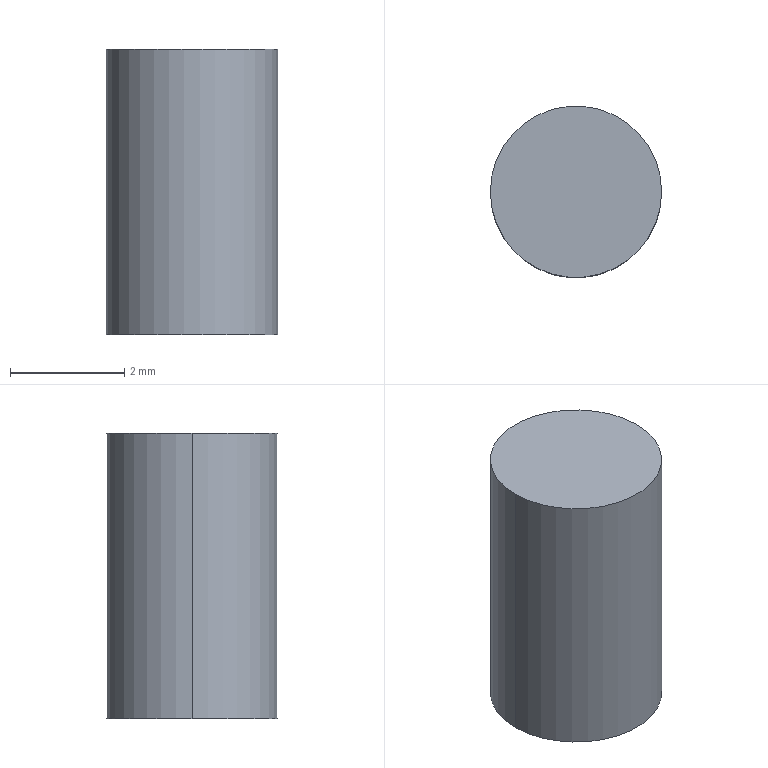Part | NX | features BREP 1 | 1 solid | 4 faces | box 3 x 3 x 5 mm | volume 35.343 mm3 | cylinder 2 | plane 2 | commonest cylinder face diameters 3 x2
STEP:
#1=CARTESIAN_POINT('',(1.5,0.,5.));
#2=VERTEX_POINT('',#1);
#3=CARTESIAN_POINT('',(-1.5,0.,5.));
#4=VERTEX_POINT('',#3);
#5=CARTESIAN_POINT('',(0.,0.,5.));
#6=DIRECTION('',(0.,0.,1.));
#7=DIRECTION('',(1.,0.,0.));
#8=AXIS2_PLACEMENT_3D('',#5,#6,#7);
#9=CIRCLE('',#8,1.5);
#10=EDGE_CURVE('',#2,#4,#9,.T.);
#11=ORIENTED_EDGE('',*,*,#10,.F.);
#12=CARTESIAN_POINT('',(1.5,0.,0.));
#13=VERTEX_POINT('',#12);
#14=CARTESIAN_POINT('',(1.5,0.,5.));
#15=DIRECTION('',(0.,0.,-1.));
#16=VECTOR('',#15,1000.);
#17=LINE('',#14,#16);
#18=EDGE_CURVE('',#2,#13,#17,.T.);
#19=ORIENTED_EDGE('',*,*,#18,.T.);
#20=CARTESIAN_POINT('',(-1.5,0.,0.));
#21=VERTEX_POINT('',#20);
#22=CARTESIAN_POINT('',(0.,0.,0.));
#23=DIRECTION('',(0.,0.,1.));
#24=DIRECTION('',(1.,0.,0.));
#25=AXIS2_PLACEMENT_3D('',#22,#23,#24);
#26=CIRCLE('',#25,1.5);
#27=EDGE_CURVE('',#13,#21,#26,.T.);
#28=ORIENTED_EDGE('',*,*,#27,.T.);
#29=CARTESIAN_POINT('',(-1.5,0.,5.));
#30=DIRECTION('',(0.,0.,-1.));
#31=VECTOR('',#30,1000.);
#32=LINE('',#29,#31);
#33=EDGE_CURVE('',#4,#21,#32,.T.);
#34=ORIENTED_EDGE('',*,*,#33,.F.);
#35=EDGE_LOOP('',(#11,#19,#28,#34));
#36=FACE_BOUND('',#35,.T.);
#37=CARTESIAN_POINT('',(0.,0.,5.));
#38=DIRECTION('',(0.,0.,-1.));
#39=DIRECTION('',(-1.,0.,0.));
#40=AXIS2_PLACEMENT_3D('',#37,#38,#39);
#41=CYLINDRICAL_SURFACE('',#40,1.5);
#42=ADVANCED_FACE('',(#36),#41,.T.);
#43=ORIENTED_EDGE('',*,*,#18,.F.);
#44=CARTESIAN_POINT('',(0.,0.,5.));
#45=DIRECTION('',(0.,0.,1.));
#46=DIRECTION('',(1.,0.,0.));
#47=AXIS2_PLACEMENT_3D('',#44,#45,#46);
#48=CIRCLE('',#47,1.5);
#49=EDGE_CURVE('',#4,#2,#48,.T.);
#50=ORIENTED_EDGE('',*,*,#49,.F.);
#51=ORIENTED_EDGE('',*,*,#33,.T.);
#52=CARTESIAN_POINT('',(0.,0.,0.));
#53=DIRECTION('',(0.,0.,1.));
#54=DIRECTION('',(1.,0.,0.));
#55=AXIS2_PLACEMENT_3D('',#52,#53,#54);
#56=CIRCLE('',#55,1.5);
#57=EDGE_CURVE('',#21,#13,#56,.T.);
#58=ORIENTED_EDGE('',*,*,#57,.T.);
#59=EDGE_LOOP('',(#43,#50,#51,#58));
#60=FACE_BOUND('',#59,.T.);
#61=CARTESIAN_POINT('',(0.,0.,5.));
#62=DIRECTION('',(0.,0.,-1.));
#63=DIRECTION('',(-1.,0.,0.));
#64=AXIS2_PLACEMENT_3D('',#61,#62,#63);
#65=CYLINDRICAL_SURFACE('',#64,1.5);
#66=ADVANCED_FACE('',(#60),#65,.T.);
#67=ORIENTED_EDGE('',*,*,#49,.T.);
#68=ORIENTED_EDGE('',*,*,#10,.T.);
#69=EDGE_LOOP('',(#67,#68));
#70=FACE_BOUND('',#69,.T.);
#71=CARTESIAN_POINT('',(0.,0.,5.));
#72=DIRECTION('',(0.,0.,1.));
#73=DIRECTION('',(1.,0.,0.));
#74=AXIS2_PLACEMENT_3D('',#71,#72,#73);
#75=PLANE('',#74);
#76=ADVANCED_FACE('',(#70),#75,.T.);
#77=ORIENTED_EDGE('',*,*,#57,.F.);
#78=ORIENTED_EDGE('',*,*,#27,.F.);
#79=EDGE_LOOP('',(#77,#78));
#80=FACE_BOUND('',#79,.T.);
#81=CARTESIAN_POINT('',(0.,0.,0.));
#82=DIRECTION('',(0.,0.,1.));
#83=DIRECTION('',(1.,0.,0.));
#84=AXIS2_PLACEMENT_3D('',#81,#82,#83);
#85=PLANE('',#84);
#86=ADVANCED_FACE('',(#80),#85,.F.);
#87=CLOSED_SHELL('',(#42,#66,#76,#86));
#88=MANIFOLD_SOLID_BREP('',#87);
#89=(LENGTH_UNIT()NAMED_UNIT(*)SI_UNIT(.MILLI.,.METRE.));
#90=UNCERTAINTY_MEASURE_WITH_UNIT(LENGTH_MEASURE(0.00001),#89,'','');
#91=(NAMED_UNIT(*)PLANE_ANGLE_UNIT()SI_UNIT($,.RADIAN.));
#92=(NAMED_UNIT(*)SI_UNIT($,.STERADIAN.)SOLID_ANGLE_UNIT());
#93=(GEOMETRIC_REPRESENTATION_CONTEXT(3)GLOBAL_UNCERTAINTY_ASSIGNED_CONTEXT((#90))GLOBAL_UNIT_ASSIGNED_CONTEXT((#89,#91,#92))REPRESENTATION_CONTEXT('',''));
#94=ADVANCED_BREP_SHAPE_REPRESENTATION('',(#88),#93);